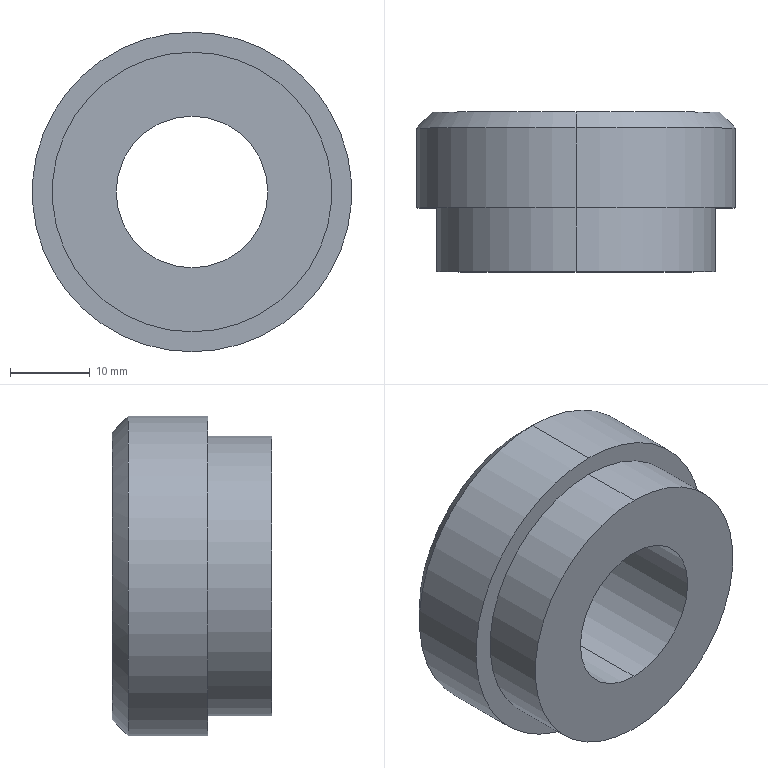Part | SolidWorks | features Chamfer 1, HoleWzd 1, Revolution 1 | 1 solid | 11 faces | box 40 x 20 x 40 mm | volume 16863 mm3 | cylinder 6 | plane 3 | cone 2 | commonest cylinder face diameters 19 x2 35 x2 40 x2
STEP:
#1=CARTESIAN_POINT('',(0.,0.,18.));
#2=VERTEX_POINT('',#1);
#3=CARTESIAN_POINT('',(0.,0.,-18.));
#4=VERTEX_POINT('',#3);
#5=CARTESIAN_POINT('',(0.,0.,0.));
#6=DIRECTION('',(0.,1.,0.));
#7=DIRECTION('',(0.,0.,1.));
#8=AXIS2_PLACEMENT_3D('',#5,#6,#7);
#9=CIRCLE('',#8,18.);
#10=EDGE_CURVE('',#2,#4,#9,.T.);
#11=ORIENTED_EDGE('',*,*,#10,.F.);
#12=CARTESIAN_POINT('',(0.,-2.,20.));
#13=VERTEX_POINT('',#12);
#14=CARTESIAN_POINT('',(0.,-2.,20.));
#15=DIRECTION('',(0.,-0.7071,0.7071));
#16=VECTOR('',#15,1000.);
#17=LINE('',#14,#16);
#18=EDGE_CURVE('',#2,#13,#17,.T.);
#19=ORIENTED_EDGE('',*,*,#18,.T.);
#20=CARTESIAN_POINT('',(0.,-2.,-20.));
#21=VERTEX_POINT('',#20);
#22=CARTESIAN_POINT('',(0.,-2.,0.));
#23=DIRECTION('',(0.,-1.,0.));
#24=DIRECTION('',(0.,0.,1.));
#25=AXIS2_PLACEMENT_3D('',#22,#23,#24);
#26=CIRCLE('',#25,20.);
#27=EDGE_CURVE('',#21,#13,#26,.T.);
#28=ORIENTED_EDGE('',*,*,#27,.F.);
#29=CARTESIAN_POINT('',(0.,-2.,-20.));
#30=DIRECTION('',(0.,-0.7071,-0.7071));
#31=VECTOR('',#30,1000.);
#32=LINE('',#29,#31);
#33=EDGE_CURVE('',#4,#21,#32,.T.);
#34=ORIENTED_EDGE('',*,*,#33,.F.);
#35=EDGE_LOOP('',(#11,#19,#28,#34));
#36=FACE_OUTER_BOUND('',#35,.T.);
#37=CARTESIAN_POINT('',(0.,-2.,0.));
#38=DIRECTION('',(0.,-1.,0.));
#39=DIRECTION('',(0.,0.,-1.));
#40=AXIS2_PLACEMENT_3D('',#37,#38,#39);
#41=CONICAL_SURFACE('',#40,20.,0.7854);
#42=ADVANCED_FACE('',(#36),#41,.T.);
#43=CARTESIAN_POINT('',(0.,-20.,9.5));
#44=VERTEX_POINT('',#43);
#45=CARTESIAN_POINT('',(0.,-20.,-9.5));
#46=VERTEX_POINT('',#45);
#47=CARTESIAN_POINT('',(0.,-20.,0.));
#48=DIRECTION('',(0.,-1.,0.));
#49=DIRECTION('',(0.,0.,-1.));
#50=AXIS2_PLACEMENT_3D('',#47,#48,#49);
#51=CIRCLE('',#50,9.5);
#52=EDGE_CURVE('',#44,#46,#51,.T.);
#53=ORIENTED_EDGE('',*,*,#52,.T.);
#54=CARTESIAN_POINT('',(0.,0.,-9.5));
#55=VERTEX_POINT('',#54);
#56=CARTESIAN_POINT('',(0.,0.,-9.5));
#57=DIRECTION('',(0.,1.,0.));
#58=VECTOR('',#57,1000.);
#59=LINE('',#56,#58);
#60=EDGE_CURVE('',#46,#55,#59,.T.);
#61=ORIENTED_EDGE('',*,*,#60,.T.);
#62=CARTESIAN_POINT('',(0.,0.,9.5));
#63=VERTEX_POINT('',#62);
#64=CARTESIAN_POINT('',(0.,0.,0.));
#65=DIRECTION('',(0.,1.,0.));
#66=DIRECTION('',(0.,0.,1.));
#67=AXIS2_PLACEMENT_3D('',#64,#65,#66);
#68=CIRCLE('',#67,9.5);
#69=EDGE_CURVE('',#55,#63,#68,.T.);
#70=ORIENTED_EDGE('',*,*,#69,.T.);
#71=CARTESIAN_POINT('',(0.,0.,9.5));
#72=DIRECTION('',(0.,1.,0.));
#73=VECTOR('',#72,1000.);
#74=LINE('',#71,#73);
#75=EDGE_CURVE('',#44,#63,#74,.T.);
#76=ORIENTED_EDGE('',*,*,#75,.F.);
#77=EDGE_LOOP('',(#53,#61,#70,#76));
#78=FACE_OUTER_BOUND('',#77,.T.);
#79=CARTESIAN_POINT('',(0.,0.,0.));
#80=DIRECTION('',(0.,1.,0.));
#81=DIRECTION('',(0.,0.,1.));
#82=AXIS2_PLACEMENT_3D('',#79,#80,#81);
#83=CYLINDRICAL_SURFACE('',#82,9.5);
#84=ADVANCED_FACE('',(#78),#83,.F.);
#85=CARTESIAN_POINT('',(0.,-12.,-17.5));
#86=VERTEX_POINT('',#85);
#87=CARTESIAN_POINT('',(0.,-12.,17.5));
#88=VERTEX_POINT('',#87);
#89=CARTESIAN_POINT('',(0.,-12.,0.));
#90=DIRECTION('',(0.,-1.,0.));
#91=DIRECTION('',(0.,0.,-1.));
#92=AXIS2_PLACEMENT_3D('',#89,#90,#91);
#93=CIRCLE('',#92,17.5);
#94=EDGE_CURVE('',#86,#88,#93,.T.);
#95=ORIENTED_EDGE('',*,*,#94,.T.);
#96=CARTESIAN_POINT('',(0.,-20.,17.5));
#97=VERTEX_POINT('',#96);
#98=CARTESIAN_POINT('',(0.,-20.,17.5));
#99=DIRECTION('',(0.,-1.,0.));
#100=VECTOR('',#99,1000.);
#101=LINE('',#98,#100);
#102=EDGE_CURVE('',#88,#97,#101,.T.);
#103=ORIENTED_EDGE('',*,*,#102,.T.);
#104=CARTESIAN_POINT('',(0.,-20.,-17.5));
#105=VERTEX_POINT('',#104);
#106=CARTESIAN_POINT('',(0.,-20.,0.));
#107=DIRECTION('',(0.,-1.,0.));
#108=DIRECTION('',(0.,0.,-1.));
#109=AXIS2_PLACEMENT_3D('',#106,#107,#108);
#110=CIRCLE('',#109,17.5);
#111=EDGE_CURVE('',#105,#97,#110,.T.);
#112=ORIENTED_EDGE('',*,*,#111,.F.);
#113=CARTESIAN_POINT('',(0.,-20.,-17.5));
#114=DIRECTION('',(0.,-1.,0.));
#115=VECTOR('',#114,1000.);
#116=LINE('',#113,#115);
#117=EDGE_CURVE('',#86,#105,#116,.T.);
#118=ORIENTED_EDGE('',*,*,#117,.F.);
#119=EDGE_LOOP('',(#95,#103,#112,#118));
#120=FACE_OUTER_BOUND('',#119,.T.);
#121=CARTESIAN_POINT('',(0.,-20.,0.));
#122=DIRECTION('',(0.,-1.,0.));
#123=DIRECTION('',(0.,0.,-1.));
#124=AXIS2_PLACEMENT_3D('',#121,#122,#123);
#125=CYLINDRICAL_SURFACE('',#124,17.5);
#126=ADVANCED_FACE('',(#120),#125,.T.);
#127=ORIENTED_EDGE('',*,*,#27,.T.);
#128=CARTESIAN_POINT('',(0.,-12.,20.));
#129=VERTEX_POINT('',#128);
#130=CARTESIAN_POINT('',(0.,-20.,20.));
#131=DIRECTION('',(0.,-1.,0.));
#132=VECTOR('',#131,1000.);
#133=LINE('',#130,#132);
#134=EDGE_CURVE('',#13,#129,#133,.T.);
#135=ORIENTED_EDGE('',*,*,#134,.T.);
#136=CARTESIAN_POINT('',(0.,-12.,-20.));
#137=VERTEX_POINT('',#136);
#138=CARTESIAN_POINT('',(0.,-12.,0.));
#139=DIRECTION('',(0.,-1.,0.));
#140=DIRECTION('',(0.,0.,-1.));
#141=AXIS2_PLACEMENT_3D('',#138,#139,#140);
#142=CIRCLE('',#141,20.);
#143=EDGE_CURVE('',#137,#129,#142,.T.);
#144=ORIENTED_EDGE('',*,*,#143,.F.);
#145=CARTESIAN_POINT('',(0.,-20.,-20.));
#146=DIRECTION('',(0.,-1.,0.));
#147=VECTOR('',#146,1000.);
#148=LINE('',#145,#147);
#149=EDGE_CURVE('',#21,#137,#148,.T.);
#150=ORIENTED_EDGE('',*,*,#149,.F.);
#151=EDGE_LOOP('',(#127,#135,#144,#150));
#152=FACE_OUTER_BOUND('',#151,.T.);
#153=CARTESIAN_POINT('',(0.,-20.,0.));
#154=DIRECTION('',(0.,-1.,0.));
#155=DIRECTION('',(0.,0.,-1.));
#156=AXIS2_PLACEMENT_3D('',#153,#154,#155);
#157=CYLINDRICAL_SURFACE('',#156,20.);
#158=ADVANCED_FACE('',(#152),#157,.T.);
#159=CARTESIAN_POINT('',(0.,0.,0.));
#160=DIRECTION('',(0.,1.,0.));
#161=DIRECTION('',(0.,0.,1.));
#162=AXIS2_PLACEMENT_3D('',#159,#160,#161);
#163=CIRCLE('',#162,18.);
#164=EDGE_CURVE('',#4,#2,#163,.T.);
#165=ORIENTED_EDGE('',*,*,#164,.T.);
#166=ORIENTED_EDGE('',*,*,#10,.T.);
#167=EDGE_LOOP('',(#165,#166));
#168=FACE_OUTER_BOUND('',#167,.T.);
#169=CARTESIAN_POINT('',(0.,0.,0.));
#170=DIRECTION('',(0.,1.,0.));
#171=DIRECTION('',(0.,0.,1.));
#172=AXIS2_PLACEMENT_3D('',#169,#170,#171);
#173=CIRCLE('',#172,9.5);
#174=EDGE_CURVE('',#63,#55,#173,.T.);
#175=ORIENTED_EDGE('',*,*,#174,.F.);
#176=ORIENTED_EDGE('',*,*,#69,.F.);
#177=EDGE_LOOP('',(#175,#176));
#178=FACE_BOUND('',#177,.T.);
#179=CARTESIAN_POINT('',(0.,0.,0.));
#180=DIRECTION('',(0.,1.,0.));
#181=DIRECTION('',(0.,0.,1.));
#182=AXIS2_PLACEMENT_3D('',#179,#180,#181);
#183=PLANE('',#182);
#184=ADVANCED_FACE('',(#168,#178),#183,.T.);
#185=ORIENTED_EDGE('',*,*,#134,.F.);
#186=CARTESIAN_POINT('',(0.,-2.,0.));
#187=DIRECTION('',(0.,-1.,0.));
#188=DIRECTION('',(0.,0.,1.));
#189=AXIS2_PLACEMENT_3D('',#186,#187,#188);
#190=CIRCLE('',#189,20.);
#191=EDGE_CURVE('',#13,#21,#190,.T.);
#192=ORIENTED_EDGE('',*,*,#191,.T.);
#193=ORIENTED_EDGE('',*,*,#149,.T.);
#194=CARTESIAN_POINT('',(0.,-12.,0.));
#195=DIRECTION('',(0.,-1.,0.));
#196=DIRECTION('',(0.,0.,-1.));
#197=AXIS2_PLACEMENT_3D('',#194,#195,#196);
#198=CIRCLE('',#197,20.);
#199=EDGE_CURVE('',#129,#137,#198,.T.);
#200=ORIENTED_EDGE('',*,*,#199,.F.);
#201=EDGE_LOOP('',(#185,#192,#193,#200));
#202=FACE_OUTER_BOUND('',#201,.T.);
#203=CARTESIAN_POINT('',(0.,-20.,0.));
#204=DIRECTION('',(0.,-1.,0.));
#205=DIRECTION('',(0.,0.,-1.));
#206=AXIS2_PLACEMENT_3D('',#203,#204,#205);
#207=CYLINDRICAL_SURFACE('',#206,20.);
#208=ADVANCED_FACE('',(#202),#207,.T.);
#209=ORIENTED_EDGE('',*,*,#143,.T.);
#210=ORIENTED_EDGE('',*,*,#199,.T.);
#211=EDGE_LOOP('',(#209,#210));
#212=FACE_OUTER_BOUND('',#211,.T.);
#213=ORIENTED_EDGE('',*,*,#94,.F.);
#214=CARTESIAN_POINT('',(0.,-12.,0.));
#215=DIRECTION('',(0.,-1.,0.));
#216=DIRECTION('',(0.,0.,-1.));
#217=AXIS2_PLACEMENT_3D('',#214,#215,#216);
#218=CIRCLE('',#217,17.5);
#219=EDGE_CURVE('',#88,#86,#218,.T.);
#220=ORIENTED_EDGE('',*,*,#219,.F.);
#221=EDGE_LOOP('',(#213,#220));
#222=FACE_BOUND('',#221,.T.);
#223=CARTESIAN_POINT('',(20.,-12.,0.));
#224=DIRECTION('',(0.,-1.,0.));
#225=DIRECTION('',(0.,0.,-1.));
#226=AXIS2_PLACEMENT_3D('',#223,#224,#225);
#227=PLANE('',#226);
#228=ADVANCED_FACE('',(#212,#222),#227,.T.);
#229=ORIENTED_EDGE('',*,*,#102,.F.);
#230=ORIENTED_EDGE('',*,*,#219,.T.);
#231=ORIENTED_EDGE('',*,*,#117,.T.);
#232=CARTESIAN_POINT('',(0.,-20.,0.));
#233=DIRECTION('',(0.,-1.,0.));
#234=DIRECTION('',(0.,0.,-1.));
#235=AXIS2_PLACEMENT_3D('',#232,#233,#234);
#236=CIRCLE('',#235,17.5);
#237=EDGE_CURVE('',#97,#105,#236,.T.);
#238=ORIENTED_EDGE('',*,*,#237,.F.);
#239=EDGE_LOOP('',(#229,#230,#231,#238));
#240=FACE_OUTER_BOUND('',#239,.T.);
#241=CARTESIAN_POINT('',(0.,-20.,0.));
#242=DIRECTION('',(0.,-1.,0.));
#243=DIRECTION('',(0.,0.,-1.));
#244=AXIS2_PLACEMENT_3D('',#241,#242,#243);
#245=CYLINDRICAL_SURFACE('',#244,17.5);
#246=ADVANCED_FACE('',(#240),#245,.T.);
#247=ORIENTED_EDGE('',*,*,#52,.F.);
#248=CARTESIAN_POINT('',(0.,-20.,0.));
#249=DIRECTION('',(0.,-1.,0.));
#250=DIRECTION('',(0.,0.,-1.));
#251=AXIS2_PLACEMENT_3D('',#248,#249,#250);
#252=CIRCLE('',#251,9.5);
#253=EDGE_CURVE('',#46,#44,#252,.T.);
#254=ORIENTED_EDGE('',*,*,#253,.F.);
#255=EDGE_LOOP('',(#247,#254));
#256=FACE_BOUND('',#255,.T.);
#257=ORIENTED_EDGE('',*,*,#111,.T.);
#258=ORIENTED_EDGE('',*,*,#237,.T.);
#259=EDGE_LOOP('',(#257,#258));
#260=FACE_OUTER_BOUND('',#259,.T.);
#261=CARTESIAN_POINT('',(17.5,-20.,0.));
#262=DIRECTION('',(0.,-1.,0.));
#263=DIRECTION('',(0.,0.,-1.));
#264=AXIS2_PLACEMENT_3D('',#261,#262,#263);
#265=PLANE('',#264);
#266=ADVANCED_FACE('',(#256,#260),#265,.T.);
#267=ORIENTED_EDGE('',*,*,#60,.F.);
#268=ORIENTED_EDGE('',*,*,#253,.T.);
#269=ORIENTED_EDGE('',*,*,#75,.T.);
#270=ORIENTED_EDGE('',*,*,#174,.T.);
#271=EDGE_LOOP('',(#267,#268,#269,#270));
#272=FACE_OUTER_BOUND('',#271,.T.);
#273=CARTESIAN_POINT('',(0.,0.,0.));
#274=DIRECTION('',(0.,1.,0.));
#275=DIRECTION('',(0.,0.,1.));
#276=AXIS2_PLACEMENT_3D('',#273,#274,#275);
#277=CYLINDRICAL_SURFACE('',#276,9.5);
#278=ADVANCED_FACE('',(#272),#277,.F.);
#279=ORIENTED_EDGE('',*,*,#18,.F.);
#280=ORIENTED_EDGE('',*,*,#164,.F.);
#281=ORIENTED_EDGE('',*,*,#33,.T.);
#282=ORIENTED_EDGE('',*,*,#191,.F.);
#283=EDGE_LOOP('',(#279,#280,#281,#282));
#284=FACE_OUTER_BOUND('',#283,.T.);
#285=CARTESIAN_POINT('',(0.,-2.,0.));
#286=DIRECTION('',(0.,-1.,0.));
#287=DIRECTION('',(0.,0.,-1.));
#288=AXIS2_PLACEMENT_3D('',#285,#286,#287);
#289=CONICAL_SURFACE('',#288,20.,0.7854);
#290=ADVANCED_FACE('',(#284),#289,.T.);
#291=CLOSED_SHELL('',(#42,#84,#126,#158,#184,#208,#228,#246,#266,#278,#290));
#292=MANIFOLD_SOLID_BREP('',#291);
#293=CARTESIAN_POINT('',(0.,0.,0.));
#294=DIRECTION('',(0.,0.,1.));
#295=DIRECTION('',(1.,0.,0.));
#296=AXIS2_PLACEMENT_3D('',#293,#294,#295);
#297=(LENGTH_UNIT()NAMED_UNIT(*)SI_UNIT(.MILLI.,.METRE.));
#298=UNCERTAINTY_MEASURE_WITH_UNIT(LENGTH_MEASURE(0.00001),#297,'','');
#299=(NAMED_UNIT(*)PLANE_ANGLE_UNIT()SI_UNIT($,.RADIAN.));
#300=(NAMED_UNIT(*)SI_UNIT($,.STERADIAN.)SOLID_ANGLE_UNIT());
#301=(GEOMETRIC_REPRESENTATION_CONTEXT(3)GLOBAL_UNCERTAINTY_ASSIGNED_CONTEXT((#298))GLOBAL_UNIT_ASSIGNED_CONTEXT((#297,#299,#300))REPRESENTATION_CONTEXT('',''));
#302=ADVANCED_BREP_SHAPE_REPRESENTATION('',(#292,#296),#301);